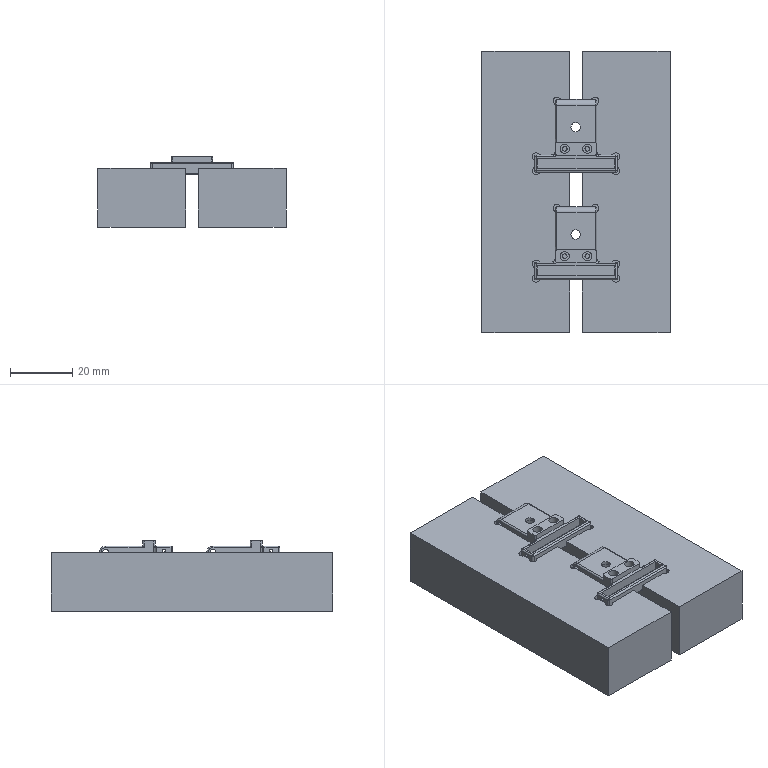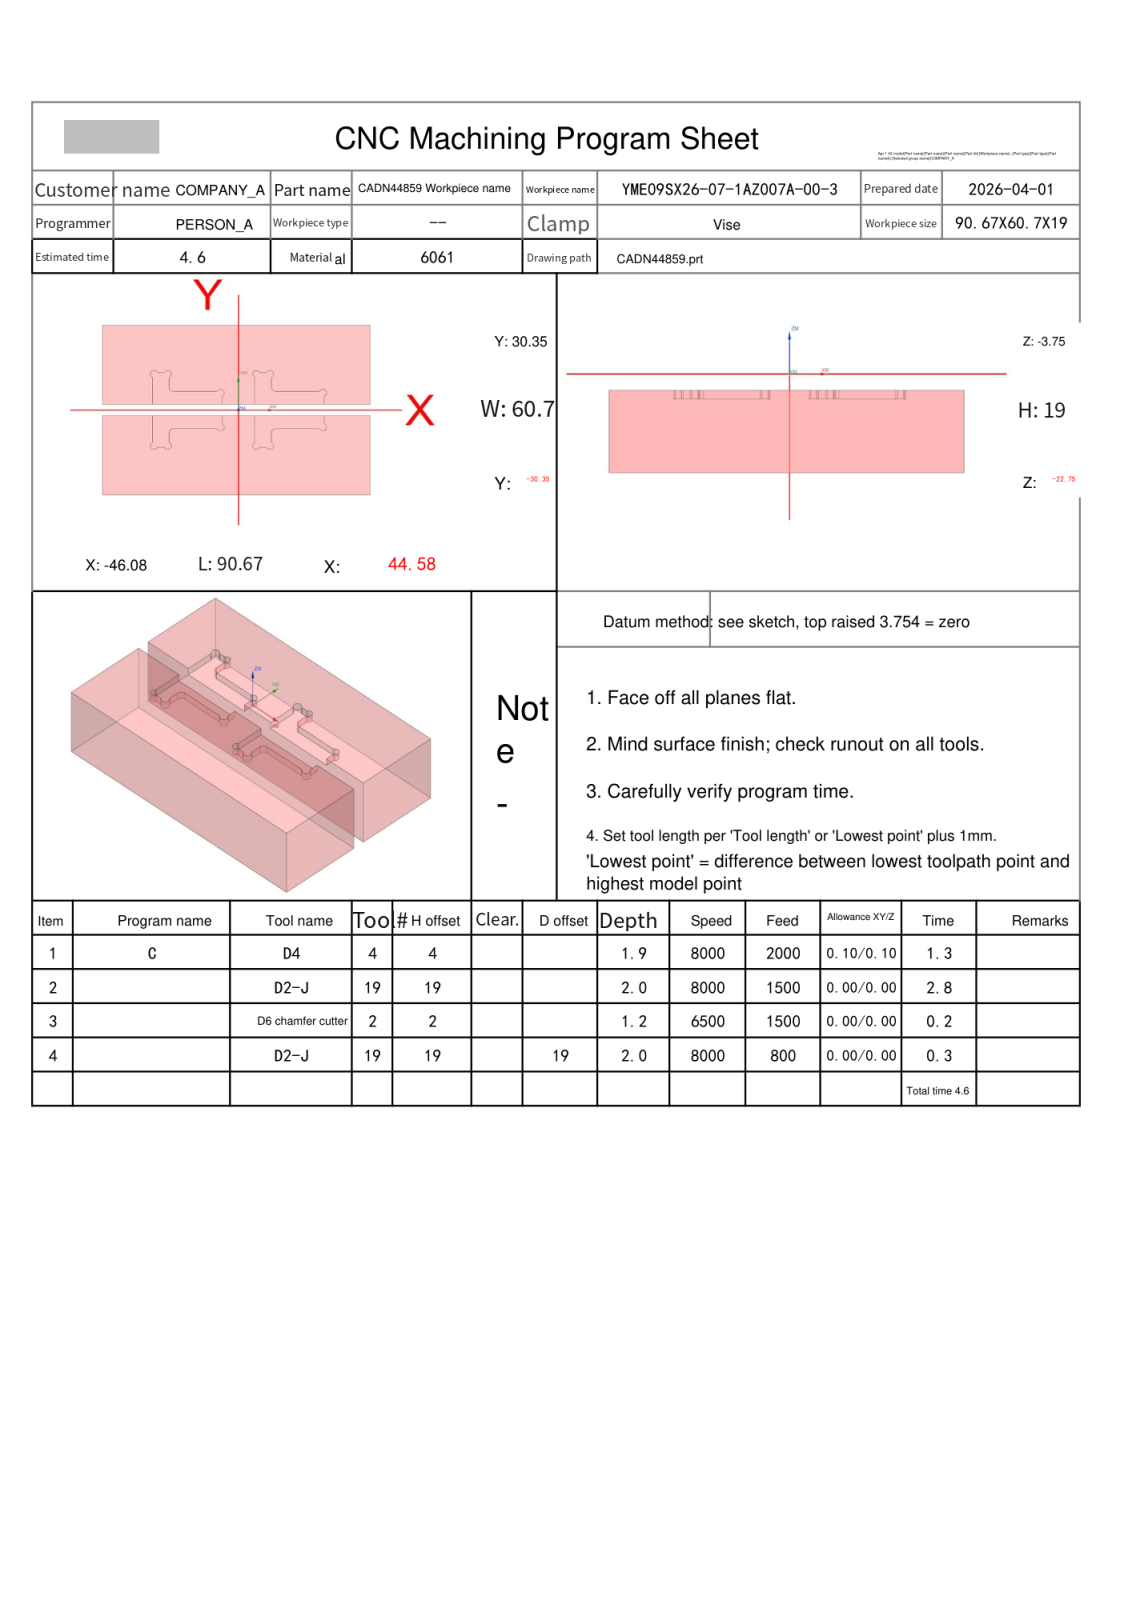NC program | NX | posted by the shop | part box 60.696 x 90.669 x 22.754 mm
Lines 1 to 949 of 8014:
%
O0001
(Machine time: 5.21 MIN)
(===Total Tool:3===)
(T4=D4      D=4.   R=0.   D-  H04 Z=-5.65 )
(T19=D2-J   D=2.   R=0.   D-  H19 Z=-5.75 )
(T2=D6 chamfer cutter   D=6.   R=0.   D-  H02 Z=-4.95 )
G80 G90 G17 G49 G40
G91 G28 Z0
M01
N1 T04 M06
(D4  D=4. R=0. H=04 ce=0.10 di=0.10)
G00 G90 G54 X-16.612 Y1.529 M03 S8000
G43 H04 Z6.346
M08
Z-2.254
G03 X-16.612 Y1.529 Z-2.847 I.128 J-1.795 F2000.
X-16.612 Y1.529 Z-3.439 I.128 J-1.795
X-16.484 Y1.534 Z-4.025 I.128 J-1.795
G01 X-21.952
G02 X-23.492 Y1.716 I0.0 J6.6
G01 X-23.584 Y1.727
G03 X-23.984 Y1.328 I0.0 J-.4
G01 Y-1.328
G03 X-23.584 Y-1.727 I.4 J.001
G01 X-23.492 Y-1.716
G02 X-21.952 Y-1.534 I1.54 J-6.418
G01 X-11.015
G03 X-10.616 Y-1.135 I-.001 J.4
G01 Y1.135
G03 X-11.015 Y1.534 I-.4 J-.001
G01 X-15.27
G02 X-15.602 Y1.712 I0.0 J.4
G01 X-17.365 Y4.356
G03 X-17.697 Y4.534 I-.333 J-.222
G01 X-21.952
G02 X-25.552 Y8.134 I0.0 J3.6
G01 Y11.248
X-26.984
Y3.819
G03 X-26.589 Y3.423 I.396 J0.0
G01 X-26.489 Y3.436
X-26.468 Y3.441
X-26.368 Y3.454
G02 X-26.013 Y3.238 I0.0 J-.4
G01 X-25.375 Y2.004
G03 X-24.487 Y1.463 I.888 J.459
X-23.487 Y2.463 I0.0 J1.
X-23.598 Y2.922 I-1. J0.0
G01 X-24.537 Y4.738
G03 X-25.425 Y5.279 I-.888 J-.459
X-26.422 Y4.365 I0.0 J-1.
G02 X-26.668 Y4.06 I-.348 J.03
G01 X-26.846 Y4.006
G03 X-26.984 Y3.819 I.057 J-.187
G01 Y-3.819
G03 X-26.846 Y-4.006 I.196 J0.0
G01 X-26.7 Y-4.051
G02 X-26.419 Y-4.389 I-.117 J-.383
G03 X-25.425 Y-5.279 I.994 J.11
X-24.537 Y-4.738 I0.0 J1.
G01 X-23.598 Y-2.922
G03 X-23.487 Y-2.463 I-.888 J.459
X-24.487 Y-1.463 I-1. J0.0
X-25.375 Y-2.004 I0.0 J-1.
G01 X-26.013 Y-3.238
G02 X-26.368 Y-3.454 I-.355 J.184
G01 X-26.468 Y-3.441
X-26.489 Y-3.436
X-26.589 Y-3.423
G03 X-26.984 Y-3.819 I0.0 J-.396
G01 Y-11.248
X-25.552
Y-8.134
G02 X-21.952 Y-4.534 I3.6 J0.0
G01 X-7.616
Y4.534
X-18.484
X-18.984
Y1.534
Z-2.525
G00 X-16.612 Y1.529
G03 X-16.612 Y1.529 Z-3.118 I.128 J-1.795
X-16.612 Y1.529 Z-3.711 I.128 J-1.795
X-16.484 Y1.534 Z-4.297 I.128 J-1.795
G01 X-21.952
G02 X-23.492 Y1.716 I0.0 J6.6
G01 X-23.584 Y1.727
G03 X-23.984 Y1.328 I0.0 J-.4
G01 Y-1.328
G03 X-23.584 Y-1.727 I.4 J.001
G01 X-23.492 Y-1.716
G02 X-21.952 Y-1.534 I1.54 J-6.418
G01 X-11.015
G03 X-10.616 Y-1.135 I-.001 J.4
G01 Y1.135
G03 X-11.015 Y1.534 I-.4 J-.001
G01 X-15.27
G02 X-15.602 Y1.712 I0.0 J.4
G01 X-17.365 Y4.356
G03 X-17.697 Y4.534 I-.333 J-.222
G01 X-21.952
G02 X-25.552 Y8.134 I0.0 J3.6
G01 Y11.248
X-26.984
Y3.819
G03 X-26.589 Y3.423 I.396 J0.0
G01 X-26.489 Y3.436
X-26.468 Y3.441
X-26.368 Y3.454
G02 X-26.013 Y3.238 I0.0 J-.4
G01 X-25.375 Y2.004
G03 X-24.487 Y1.463 I.888 J.459
X-23.487 Y2.463 I0.0 J1.
X-23.598 Y2.922 I-1. J0.0
G01 X-24.537 Y4.738
G03 X-25.425 Y5.279 I-.888 J-.459
X-26.422 Y4.365 I0.0 J-1.
G02 X-26.668 Y4.06 I-.348 J.03
G01 X-26.846 Y4.006
G03 X-26.984 Y3.819 I.057 J-.187
G01 Y-3.819
G03 X-26.846 Y-4.006 I.196 J0.0
G01 X-26.7 Y-4.051
G02 X-26.419 Y-4.389 I-.117 J-.383
G03 X-25.425 Y-5.279 I.994 J.11
X-24.537 Y-4.738 I0.0 J1.
G01 X-23.598 Y-2.922
G03 X-23.487 Y-2.463 I-.888 J.459
X-24.487 Y-1.463 I-1. J0.0
X-25.375 Y-2.004 I0.0 J-1.
G01 X-26.013 Y-3.238
G02 X-26.368 Y-3.454 I-.355 J.184
G01 X-26.468 Y-3.441
X-26.489 Y-3.436
X-26.589 Y-3.423
G03 X-26.984 Y-3.819 I0.0 J-.396
G01 Y-11.248
X-25.552
Y-8.134
G02 X-21.952 Y-4.534 I3.6 J0.0
G01 X-7.616
Y4.534
X-18.484
X-18.984
Y1.534
Z-2.797
G00 X-16.612 Y1.529
G03 X-16.612 Y1.529 Z-3.39 I.128 J-1.795
X-16.612 Y1.529 Z-3.982 I.128 J-1.795
X-16.484 Y1.534 Z-4.568 I.128 J-1.795
G01 X-21.952
G02 X-23.492 Y1.716 I0.0 J6.6
G01 X-23.584 Y1.727
G03 X-23.984 Y1.328 I0.0 J-.4
G01 Y-1.328
G03 X-23.584 Y-1.727 I.4 J.001
G01 X-23.492 Y-1.716
G02 X-21.952 Y-1.534 I1.54 J-6.418
G01 X-11.015
G03 X-10.616 Y-1.135 I-.001 J.4
G01 Y1.135
G03 X-11.015 Y1.534 I-.4 J-.001
G01 X-15.27
G02 X-15.602 Y1.712 I0.0 J.4
G01 X-17.365 Y4.356
G03 X-17.697 Y4.534 I-.333 J-.222
G01 X-21.952
G02 X-25.552 Y8.134 I0.0 J3.6
G01 Y11.248
X-26.984
Y3.819
G03 X-26.589 Y3.423 I.396 J0.0
G01 X-26.489 Y3.436
X-26.468 Y3.441
X-26.368 Y3.454
G02 X-26.013 Y3.238 I0.0 J-.4
G01 X-25.375 Y2.004
G03 X-24.487 Y1.463 I.888 J.459
X-23.487 Y2.463 I0.0 J1.
X-23.598 Y2.922 I-1. J0.0
G01 X-24.537 Y4.738
G03 X-25.425 Y5.279 I-.888 J-.459
X-26.422 Y4.365 I0.0 J-1.
G02 X-26.668 Y4.06 I-.348 J.03
G01 X-26.846 Y4.006
G03 X-26.984 Y3.819 I.057 J-.187
G01 Y-3.819
G03 X-26.846 Y-4.006 I.196 J0.0
G01 X-26.7 Y-4.051
G02 X-26.419 Y-4.389 I-.117 J-.383
G03 X-25.425 Y-5.279 I.994 J.11
X-24.537 Y-4.738 I0.0 J1.
G01 X-23.598 Y-2.922
G03 X-23.487 Y-2.463 I-.888 J.459
X-24.487 Y-1.463 I-1. J0.0
X-25.375 Y-2.004 I0.0 J-1.
G01 X-26.013 Y-3.238
G02 X-26.368 Y-3.454 I-.355 J.184
G01 X-26.468 Y-3.441
X-26.489 Y-3.436
X-26.589 Y-3.423
G03 X-26.984 Y-3.819 I0.0 J-.396
G01 Y-11.248
X-25.552
Y-8.134
G02 X-21.952 Y-4.534 I3.6 J0.0
G01 X-7.616
Y4.534
X-18.484
X-18.984
Y1.534
Z-3.068
G00 X-16.612 Y1.529
G03 X-16.612 Y1.529 Z-3.661 I.128 J-1.795
X-16.612 Y1.529 Z-4.254 I.128 J-1.795
X-16.484 Y1.534 Z-4.84 I.128 J-1.795
G01 X-21.952
G02 X-23.492 Y1.716 I0.0 J6.6
G01 X-23.584 Y1.727
G03 X-23.984 Y1.328 I0.0 J-.4
G01 Y-1.328
G03 X-23.584 Y-1.727 I.4 J.001
G01 X-23.492 Y-1.716
G02 X-21.952 Y-1.534 I1.54 J-6.418
G01 X-11.015
G03 X-10.616 Y-1.135 I-.001 J.4
G01 Y1.135
G03 X-11.015 Y1.534 I-.4 J-.001
G01 X-15.27
G02 X-15.602 Y1.712 I0.0 J.4
G01 X-17.365 Y4.356
G03 X-17.697 Y4.534 I-.333 J-.222
G01 X-21.952
G02 X-25.552 Y8.134 I0.0 J3.6
G01 Y11.248
X-26.984
Y3.819
G03 X-26.589 Y3.423 I.396 J0.0
G01 X-26.489 Y3.436
X-26.468 Y3.441
X-26.368 Y3.454
G02 X-26.013 Y3.238 I0.0 J-.4
G01 X-25.375 Y2.004
G03 X-24.487 Y1.463 I.888 J.459
X-23.487 Y2.463 I0.0 J1.
X-23.598 Y2.922 I-1. J0.0
G01 X-24.537 Y4.738
G03 X-25.425 Y5.279 I-.888 J-.459
X-26.422 Y4.365 I0.0 J-1.
G02 X-26.668 Y4.06 I-.348 J.03
G01 X-26.846 Y4.006
G03 X-26.984 Y3.819 I.057 J-.187
G01 Y-3.819
G03 X-26.846 Y-4.006 I.196 J0.0
G01 X-26.7 Y-4.051
G02 X-26.419 Y-4.389 I-.117 J-.383
G03 X-25.425 Y-5.279 I.994 J.11
X-24.537 Y-4.738 I0.0 J1.
G01 X-23.598 Y-2.922
G03 X-23.487 Y-2.463 I-.888 J.459
X-24.487 Y-1.463 I-1. J0.0
X-25.375 Y-2.004 I0.0 J-1.
G01 X-26.013 Y-3.238
G02 X-26.368 Y-3.454 I-.355 J.184
G01 X-26.468 Y-3.441
X-26.489 Y-3.436
X-26.589 Y-3.423
G03 X-26.984 Y-3.819 I0.0 J-.396
G01 Y-11.248
X-25.552
Y-8.134
G02 X-21.952 Y-4.534 I3.6 J0.0
G01 X-7.616
Y4.534
X-18.484
X-18.984
Y1.534
Z-3.34
G00 X-16.612 Y1.529
G03 X-16.612 Y1.529 Z-3.932 I.128 J-1.795
X-16.612 Y1.529 Z-4.525 I.128 J-1.795
X-16.484 Y1.534 Z-5.111 I.128 J-1.795
G01 X-21.952
G02 X-23.492 Y1.716 I0.0 J6.6
G01 X-23.584 Y1.727
G03 X-23.984 Y1.328 I0.0 J-.4
G01 Y-1.328
G03 X-23.584 Y-1.727 I.4 J.001
G01 X-23.492 Y-1.716
G02 X-21.952 Y-1.534 I1.54 J-6.418
G01 X-11.015
G03 X-10.616 Y-1.135 I-.001 J.4
G01 Y1.135
G03 X-11.015 Y1.534 I-.4 J-.001
G01 X-15.27
G02 X-15.602 Y1.712 I0.0 J.4
G01 X-17.365 Y4.356
G03 X-17.697 Y4.534 I-.333 J-.222
G01 X-21.952
G02 X-25.552 Y8.134 I0.0 J3.6
G01 Y11.248
X-26.984
Y3.819
G03 X-26.589 Y3.423 I.396 J0.0
G01 X-26.489 Y3.436
X-26.468 Y3.441
X-26.368 Y3.454
G02 X-26.013 Y3.238 I0.0 J-.4
G01 X-25.375 Y2.004
G03 X-24.487 Y1.463 I.888 J.459
X-23.487 Y2.463 I0.0 J1.
X-23.598 Y2.922 I-1. J0.0
G01 X-24.537 Y4.738
G03 X-25.425 Y5.279 I-.888 J-.459
X-26.422 Y4.365 I0.0 J-1.
G02 X-26.668 Y4.06 I-.348 J.03
G01 X-26.846 Y4.006
G03 X-26.984 Y3.819 I.057 J-.187
G01 Y-3.819
G03 X-26.846 Y-4.006 I.196 J0.0
G01 X-26.7 Y-4.051
G02 X-26.419 Y-4.389 I-.117 J-.383
G03 X-25.425 Y-5.279 I.994 J.11
X-24.537 Y-4.738 I0.0 J1.
G01 X-23.598 Y-2.922
G03 X-23.487 Y-2.463 I-.888 J.459
X-24.487 Y-1.463 I-1. J0.0
X-25.375 Y-2.004 I0.0 J-1.
G01 X-26.013 Y-3.238
G02 X-26.368 Y-3.454 I-.355 J.184
G01 X-26.468 Y-3.441
X-26.489 Y-3.436
X-26.589 Y-3.423
G03 X-26.984 Y-3.819 I0.0 J-.396
G01 Y-11.248
X-25.552
Y-8.134
G02 X-21.952 Y-4.534 I3.6 J0.0
G01 X-7.616
Y4.534
X-18.484
X-18.984
Y1.534
Z-3.611
G00 X-16.612 Y1.529
G03 X-16.612 Y1.529 Z-4.204 I.128 J-1.795
X-16.612 Y1.529 Z-4.797 I.128 J-1.795
X-16.484 Y1.534 Z-5.383 I.128 J-1.795
G01 X-21.952
G02 X-23.492 Y1.716 I0.0 J6.6
G01 X-23.584 Y1.727
G03 X-23.984 Y1.328 I0.0 J-.4
G01 Y-1.328
G03 X-23.584 Y-1.727 I.4 J.001
G01 X-23.492 Y-1.716
G02 X-21.952 Y-1.534 I1.54 J-6.418
G01 X-11.015
G03 X-10.616 Y-1.135 I-.001 J.4
G01 Y1.135
G03 X-11.015 Y1.534 I-.4 J-.001
G01 X-15.27
G02 X-15.602 Y1.712 I0.0 J.4
G01 X-17.365 Y4.356
G03 X-17.697 Y4.534 I-.333 J-.222
G01 X-21.952
G02 X-25.552 Y8.134 I0.0 J3.6
G01 Y11.248
X-26.984
Y3.819
G03 X-26.589 Y3.423 I.396 J0.0
G01 X-26.489 Y3.436
X-26.468 Y3.441
X-26.368 Y3.454
G02 X-26.013 Y3.238 I0.0 J-.4
G01 X-25.375 Y2.004
G03 X-24.487 Y1.463 I.888 J.459
X-23.487 Y2.463 I0.0 J1.
X-23.598 Y2.922 I-1. J0.0
G01 X-24.537 Y4.738
G03 X-25.425 Y5.279 I-.888 J-.459
X-26.422 Y4.365 I0.0 J-1.
G02 X-26.668 Y4.06 I-.348 J.03
G01 X-26.846 Y4.006
G03 X-26.984 Y3.819 I.057 J-.187
G01 Y-3.819
G03 X-26.846 Y-4.006 I.196 J0.0
G01 X-26.7 Y-4.051
G02 X-26.419 Y-4.389 I-.117 J-.383
G03 X-25.425 Y-5.279 I.994 J.11
X-24.537 Y-4.738 I0.0 J1.
G01 X-23.598 Y-2.922
G03 X-23.487 Y-2.463 I-.888 J.459
X-24.487 Y-1.463 I-1. J0.0
X-25.375 Y-2.004 I0.0 J-1.
G01 X-26.013 Y-3.238
G02 X-26.368 Y-3.454 I-.355 J.184
G01 X-26.468 Y-3.441
X-26.489 Y-3.436
X-26.589 Y-3.423
G03 X-26.984 Y-3.819 I0.0 J-.396
G01 Y-11.248
X-25.552
Y-8.134
G02 X-21.952 Y-4.534 I3.6 J0.0
G01 X-7.616
Y4.534
X-18.484
X-18.984
Y1.534
Z-3.883
G00 X-16.612 Y1.529
G03 X-16.612 Y1.529 Z-4.475 I.128 J-1.795
X-16.612 Y1.529 Z-5.068 I.128 J-1.795
X-16.484 Y1.534 Z-5.654 I.128 J-1.795
G01 X-21.952
G02 X-23.492 Y1.716 I0.0 J6.6
G01 X-23.584 Y1.727
G03 X-23.984 Y1.328 I0.0 J-.4
G01 Y-1.328
G03 X-23.584 Y-1.727 I.4 J.001
G01 X-23.492 Y-1.716
G02 X-21.952 Y-1.534 I1.54 J-6.418
G01 X-11.015
G03 X-10.616 Y-1.135 I-.001 J.4
G01 Y1.135
G03 X-11.015 Y1.534 I-.4 J-.001
G01 X-15.27
G02 X-15.602 Y1.712 I0.0 J.4
G01 X-17.365 Y4.356
G03 X-17.697 Y4.534 I-.333 J-.222
G01 X-21.952
G02 X-25.552 Y8.134 I0.0 J3.6
G01 Y11.248
X-26.984
Y3.819
G03 X-26.589 Y3.423 I.396 J0.0
G01 X-26.489 Y3.436
X-26.468 Y3.441
X-26.368 Y3.454
G02 X-26.013 Y3.238 I0.0 J-.4
G01 X-25.375 Y2.004
G03 X-24.487 Y1.463 I.888 J.459
X-23.487 Y2.463 I0.0 J1.
X-23.598 Y2.922 I-1. J0.0
G01 X-24.537 Y4.738
G03 X-25.425 Y5.279 I-.888 J-.459
X-26.422 Y4.365 I0.0 J-1.
G02 X-26.668 Y4.06 I-.348 J.03
G01 X-26.846 Y4.006
G03 X-26.984 Y3.819 I.057 J-.187
G01 Y-3.819
G03 X-26.846 Y-4.006 I.196 J0.0
G01 X-26.7 Y-4.051
G02 X-26.419 Y-4.389 I-.117 J-.383
G03 X-25.425 Y-5.279 I.994 J.11
X-24.537 Y-4.738 I0.0 J1.
G01 X-23.598 Y-2.922
G03 X-23.487 Y-2.463 I-.888 J.459
X-24.487 Y-1.463 I-1. J0.0
X-25.375 Y-2.004 I0.0 J-1.
G01 X-26.013 Y-3.238
G02 X-26.368 Y-3.454 I-.355 J.184
G01 X-26.468 Y-3.441
X-26.489 Y-3.436
X-26.589 Y-3.423
G03 X-26.984 Y-3.819 I0.0 J-.396
G01 Y-11.248
X-25.552
Y-8.134
G02 X-21.952 Y-4.534 I3.6 J0.0
G01 X-7.616
Y4.534
X-18.484
X-18.984
Y1.534
Z-4.154
G00 Z6.346
X17.988 Y1.529
Z-2.254
G03 X17.988 Y1.529 Z-2.847 I.128 J-1.795
X17.988 Y1.529 Z-3.439 I.128 J-1.795
X18.116 Y1.534 Z-4.025 I.128 J-1.795
G01 X12.648
G02 X11.108 Y1.716 I0.0 J6.6
G01 X11.016 Y1.727
G03 X10.616 Y1.328 I0.0 J-.4
G01 Y-1.328
G03 X11.016 Y-1.727 I.4 J.001
G01 X11.108 Y-1.716
G02 X12.648 Y-1.534 I1.54 J-6.418
G01 X23.585
G03 X23.984 Y-1.135 I-.001 J.4
G01 Y1.135
G03 X23.585 Y1.534 I-.4 J-.001
G01 X19.33
G02 X18.998 Y1.712 I0.0 J.4
G01 X17.235 Y4.356
G03 X16.903 Y4.534 I-.333 J-.222
G01 X12.648
G02 X9.048 Y8.134 I0.0 J3.6
G01 Y11.248
X7.616
Y3.819
G03 X8.011 Y3.423 I.396 J0.0
G01 X8.111 Y3.436
X8.132 Y3.441
X8.232 Y3.454
G02 X8.587 Y3.238 I0.0 J-.4
G01 X9.225 Y2.004
G03 X10.113 Y1.463 I.888 J.459
X11.113 Y2.463 I0.0 J1.
X11.002 Y2.922 I-1. J0.0
G01 X10.063 Y4.738
G03 X9.175 Y5.279 I-.888 J-.459
X8.178 Y4.365 I0.0 J-1.
G02 X7.932 Y4.06 I-.348 J.03
G01 X7.754 Y4.006
G03 X7.616 Y3.819 I.057 J-.187
G01 Y-3.819
G03 X7.754 Y-4.006 I.196 J0.0
G01 X7.9 Y-4.051
G02 X8.181 Y-4.389 I-.117 J-.383
G03 X9.175 Y-5.279 I.994 J.11
X10.063 Y-4.738 I0.0 J1.
G01 X11.002 Y-2.922
G03 X11.113 Y-2.463 I-.888 J.459
X10.113 Y-1.463 I-1. J0.0
X9.225 Y-2.004 I0.0 J-1.
G01 X8.587 Y-3.238
G02 X8.232 Y-3.454 I-.355 J.184
G01 X8.132 Y-3.441
X8.111 Y-3.436
X8.011 Y-3.423
G03 X7.616 Y-3.819 I0.0 J-.396
G01 Y-11.248
X9.048
Y-8.134
G02 X12.648 Y-4.534 I3.6 J0.0
G01 X26.984
Y4.534
X16.116
X15.616
Y1.534
Z-2.525
G00 X17.988 Y1.529
G03 X17.988 Y1.529 Z-3.118 I.128 J-1.795
X17.988 Y1.529 Z-3.711 I.128 J-1.795
X18.116 Y1.534 Z-4.297 I.128 J-1.795
G01 X12.648
G02 X11.108 Y1.716 I0.0 J6.6
G01 X11.016 Y1.727
G03 X10.616 Y1.328 I0.0 J-.4
G01 Y-1.328
G03 X11.016 Y-1.727 I.4 J.001
G01 X11.108 Y-1.716
G02 X12.648 Y-1.534 I1.54 J-6.418
G01 X23.585
G03 X23.984 Y-1.135 I-.001 J.4
G01 Y1.135
G03 X23.585 Y1.534 I-.4 J-.001
G01 X19.33
G02 X18.998 Y1.712 I0.0 J.4
G01 X17.235 Y4.356
G03 X16.903 Y4.534 I-.333 J-.222
G01 X12.648
G02 X9.048 Y8.134 I0.0 J3.6
G01 Y11.248
X7.616
Y3.819
G03 X8.011 Y3.423 I.396 J0.0
G01 X8.111 Y3.436
X8.132 Y3.441
X8.232 Y3.454
G02 X8.587 Y3.238 I0.0 J-.4
G01 X9.225 Y2.004
G03 X10.113 Y1.463 I.888 J.459
X11.113 Y2.463 I0.0 J1.
X11.002 Y2.922 I-1. J0.0
G01 X10.063 Y4.738
G03 X9.175 Y5.279 I-.888 J-.459
X8.178 Y4.365 I0.0 J-1.
G02 X7.932 Y4.06 I-.348 J.03
G01 X7.754 Y4.006
G03 X7.616 Y3.819 I.057 J-.187
G01 Y-3.819
G03 X7.754 Y-4.006 I.196 J0.0
G01 X7.9 Y-4.051
G02 X8.181 Y-4.389 I-.117 J-.383
G03 X9.175 Y-5.279 I.994 J.11
X10.063 Y-4.738 I0.0 J1.
G01 X11.002 Y-2.922
G03 X11.113 Y-2.463 I-.888 J.459
X10.113 Y-1.463 I-1. J0.0
X9.225 Y-2.004 I0.0 J-1.
G01 X8.587 Y-3.238
G02 X8.232 Y-3.454 I-.355 J.184
G01 X8.132 Y-3.441
X8.111 Y-3.436
X8.011 Y-3.423
G03 X7.616 Y-3.819 I0.0 J-.396
G01 Y-11.248
X9.048
Y-8.134
G02 X12.648 Y-4.534 I3.6 J0.0
G01 X26.984
Y4.534
X16.116
X15.616
Y1.534
Z-2.797
G00 X17.988 Y1.529
G03 X17.988 Y1.529 Z-3.39 I.128 J-1.795
X17.988 Y1.529 Z-3.982 I.128 J-1.795
X18.116 Y1.534 Z-4.568 I.128 J-1.795
G01 X12.648
G02 X11.108 Y1.716 I0.0 J6.6
G01 X11.016 Y1.727
G03 X10.616 Y1.328 I0.0 J-.4
G01 Y-1.328
G03 X11.016 Y-1.727 I.4 J.001
G01 X11.108 Y-1.716
G02 X12.648 Y-1.534 I1.54 J-6.418
G01 X23.585
G03 X23.984 Y-1.135 I-.001 J.4
G01 Y1.135
G03 X23.585 Y1.534 I-.4 J-.001
G01 X19.33
G02 X18.998 Y1.712 I0.0 J.4
G01 X17.235 Y4.356
G03 X16.903 Y4.534 I-.333 J-.222
G01 X12.648
G02 X9.048 Y8.134 I0.0 J3.6
G01 Y11.248
X7.616
Y3.819
G03 X8.011 Y3.423 I.396 J0.0
G01 X8.111 Y3.436
X8.132 Y3.441
X8.232 Y3.454
G02 X8.587 Y3.238 I0.0 J-.4
G01 X9.225 Y2.004
G03 X10.113 Y1.463 I.888 J.459
X11.113 Y2.463 I0.0 J1.
X11.002 Y2.922 I-1. J0.0
G01 X10.063 Y4.738
G03 X9.175 Y5.279 I-.888 J-.459
X8.178 Y4.365 I0.0 J-1.
G02 X7.932 Y4.06 I-.348 J.03
G01 X7.754 Y4.006
G03 X7.616 Y3.819 I.057 J-.187
G01 Y-3.819
G03 X7.754 Y-4.006 I.196 J0.0
G01 X7.9 Y-4.051
G02 X8.181 Y-4.389 I-.117 J-.383
G03 X9.175 Y-5.279 I.994 J.11
X10.063 Y-4.738 I0.0 J1.
G01 X11.002 Y-2.922
G03 X11.113 Y-2.463 I-.888 J.459
X10.113 Y-1.463 I-1. J0.0
X9.225 Y-2.004 I0.0 J-1.
G01 X8.587 Y-3.238
G02 X8.232 Y-3.454 I-.355 J.184
G01 X8.132 Y-3.441
X8.111 Y-3.436
X8.011 Y-3.423
G03 X7.616 Y-3.819 I0.0 J-.396
G01 Y-11.248
X9.048
Y-8.134
G02 X12.648 Y-4.534 I3.6 J0.0
G01 X26.984
Y4.534
X16.116
X15.616
Y1.534
Z-3.068
G00 X17.988 Y1.529
G03 X17.988 Y1.529 Z-3.661 I.128 J-1.795
X17.988 Y1.529 Z-4.254 I.128 J-1.795
X18.116 Y1.534 Z-4.84 I.128 J-1.795
G01 X12.648
G02 X11.108 Y1.716 I0.0 J6.6
G01 X11.016 Y1.727
G03 X10.616 Y1.328 I0.0 J-.4
G01 Y-1.328
G03 X11.016 Y-1.727 I.4 J.001
G01 X11.108 Y-1.716
G02 X12.648 Y-1.534 I1.54 J-6.418
G01 X23.585
G03 X23.984 Y-1.135 I-.001 J.4
G01 Y1.135
G03 X23.585 Y1.534 I-.4 J-.001
G01 X19.33
G02 X18.998 Y1.712 I0.0 J.4
G01 X17.235 Y4.356
G03 X16.903 Y4.534 I-.333 J-.222
G01 X12.648
G02 X9.048 Y8.134 I0.0 J3.6
G01 Y11.248
X7.616
Y3.819
G03 X8.011 Y3.423 I.396 J0.0
G01 X8.111 Y3.436
X8.132 Y3.441
X8.232 Y3.454
G02 X8.587 Y3.238 I0.0 J-.4
G01 X9.225 Y2.004
G03 X10.113 Y1.463 I.888 J.459
X11.113 Y2.463 I0.0 J1.
X11.002 Y2.922 I-1. J0.0
G01 X10.063 Y4.738
G03 X9.175 Y5.279 I-.888 J-.459
X8.178 Y4.365 I0.0 J-1.
G02 X7.932 Y4.06 I-.348 J.03
G01 X7.754 Y4.006
G03 X7.616 Y3.819 I.057 J-.187
G01 Y-3.819
G03 X7.754 Y-4.006 I.196 J0.0
G01 X7.9 Y-4.051
G02 X8.181 Y-4.389 I-.117 J-.383
G03 X9.175 Y-5.279 I.994 J.11
X10.063 Y-4.738 I0.0 J1.
G01 X11.002 Y-2.922
G03 X11.113 Y-2.463 I-.888 J.459
X10.113 Y-1.463 I-1. J0.0
X9.225 Y-2.004 I0.0 J-1.
G01 X8.587 Y-3.238
G02 X8.232 Y-3.454 I-.355 J.184
G01 X8.132 Y-3.441
X8.111 Y-3.436
X8.011 Y-3.423
G03 X7.616 Y-3.819 I0.0 J-.396
G01 Y-11.248
X9.048
Y-8.134
G02 X12.648 Y-4.534 I3.6 J0.0
G01 X26.984
Y4.534
X16.116
X15.616
Y1.534
Z-3.34
G00 X17.988 Y1.529
G03 X17.988 Y1.529 Z-3.932 I.128 J-1.795
X17.988 Y1.529 Z-4.525 I.128 J-1.795
X18.116 Y1.534 Z-5.111 I.128 J-1.795
G01 X12.648
G02 X11.108 Y1.716 I0.0 J6.6
G01 X11.016 Y1.727
G03 X10.616 Y1.328 I0.0 J-.4
G01 Y-1.328
G03 X11.016 Y-1.727 I.4 J.001
G01 X11.108 Y-1.716
G02 X12.648 Y-1.534 I1.54 J-6.418
G01 X23.585
G03 X23.984 Y-1.135 I-.001 J.4
G01 Y1.135
G03 X23.585 Y1.534 I-.4 J-.001
G01 X19.33
G02 X18.998 Y1.712 I0.0 J.4
G01 X17.235 Y4.356
G03 X16.903 Y4.534 I-.333 J-.222
G01 X12.648
G02 X9.048 Y8.134 I0.0 J3.6
G01 Y11.248
X7.616
Y3.819
G03 X8.011 Y3.423 I.396 J0.0
G01 X8.111 Y3.436
X8.132 Y3.441
X8.232 Y3.454
G02 X8.587 Y3.238 I0.0 J-.4
G01 X9.225 Y2.004
G03 X10.113 Y1.463 I.888 J.459
X11.113 Y2.463 I0.0 J1.
X11.002 Y2.922 I-1. J0.0
G01 X10.063 Y4.738
G03 X9.175 Y5.279 I-.888 J-.459
X8.178 Y4.365 I0.0 J-1.
G02 X7.932 Y4.06 I-.348 J.03
G01 X7.754 Y4.006
G03 X7.616 Y3.819 I.057 J-.187
G01 Y-3.819
G03 X7.754 Y-4.006 I.196 J0.0
G01 X7.9 Y-4.051
G02 X8.181 Y-4.389 I-.117 J-.383
G03 X9.175 Y-5.279 I.994 J.11
X10.063 Y-4.738 I0.0 J1.
G01 X11.002 Y-2.922
G03 X11.113 Y-2.463 I-.888 J.459
X10.113 Y-1.463 I-1. J0.0
X9.225 Y-2.004 I0.0 J-1.
G01 X8.587 Y-3.238
G02 X8.232 Y-3.454 I-.355 J.184
G01 X8.132 Y-3.441
X8.111 Y-3.436
X8.011 Y-3.423
G03 X7.616 Y-3.819 I0.0 J-.396
G01 Y-11.248
X9.048
Y-8.134
G02 X12.648 Y-4.534 I3.6 J0.0
G01 X26.984
Y4.534
X16.116
X15.616
Y1.534
Z-3.611
G00 X17.988 Y1.529
G03 X17.988 Y1.529 Z-4.204 I.128 J-1.795
X17.988 Y1.529 Z-4.797 I.128 J-1.795
X18.116 Y1.534 Z-5.383 I.128 J-1.795
G01 X12.648
G02 X11.108 Y1.716 I0.0 J6.6
G01 X11.016 Y1.727
G03 X10.616 Y1.328 I0.0 J-.4
G01 Y-1.328
G03 X11.016 Y-1.727 I.4 J.001
G01 X11.108 Y-1.716
G02 X12.648 Y-1.534 I1.54 J-6.418
G01 X23.585
G03 X23.984 Y-1.135 I-.001 J.4
G01 Y1.135
G03 X23.585 Y1.534 I-.4 J-.001
G01 X19.33
G02 X18.998 Y1.712 I0.0 J.4
G01 X17.235 Y4.356
G03 X16.903 Y4.534 I-.333 J-.222
G01 X12.648
G02 X9.048 Y8.134 I0.0 J3.6
G01 Y11.248
X7.616
Y3.819
G03 X8.011 Y3.423 I.396 J0.0
G01 X8.111 Y3.436
X8.132 Y3.441
X8.232 Y3.454
G02 X8.587 Y3.238 I0.0 J-.4
G01 X9.225 Y2.004
G03 X10.113 Y1.463 I.888 J.459
X11.113 Y2.463 I0.0 J1.
X11.002 Y2.922 I-1. J0.0
G01 X10.063 Y4.738
G03 X9.175 Y5.279 I-.888 J-.459
X8.178 Y4.365 I0.0 J-1.
G02 X7.932 Y4.06 I-.348 J.03
G01 X7.754 Y4.006
G03 X7.616 Y3.819 I.057 J-.187
G01 Y-3.819
G03 X7.754 Y-4.006 I.196 J0.0
G01 X7.9 Y-4.051
G02 X8.181 Y-4.389 I-.117 J-.383
G03 X9.175 Y-5.279 I.994 J.11
X10.063 Y-4.738 I0.0 J1.
G01 X11.002 Y-2.922
G03 X11.113 Y-2.463 I-.888 J.459
X10.113 Y-1.463 I-1. J0.0
X9.225 Y-2.004 I0.0 J-1.
G01 X8.587 Y-3.238
G02 X8.232 Y-3.454 I-.355 J.184
G01 X8.132 Y-3.441
X8.111 Y-3.436
X8.011 Y-3.423
G03 X7.616 Y-3.819 I0.0 J-.396
G01 Y-11.248
X9.048
Y-8.134
G02 X12.648 Y-4.534 I3.6 J0.0
G01 X26.984
Y4.534
X16.116
X15.616
Y1.534
Z-3.883
G00 X17.988 Y1.529
G03 X17.988 Y1.529 Z-4.475 I.128 J-1.795
X17.988 Y1.529 Z-5.068 I.128 J-1.795
X18.116 Y1.534 Z-5.654 I.128 J-1.795
G01 X12.648
G02 X11.108 Y1.716 I0.0 J6.6
G01 X11.016 Y1.727
G03 X10.616 Y1.328 I0.0 J-.4
G01 Y-1.328
G03 X11.016 Y-1.727 I.4 J.001
G01 X11.108 Y-1.716
G02 X12.648 Y-1.534 I1.54 J-6.418
G01 X23.585
G03 X23.984 Y-1.135 I-.001 J.4
G01 Y1.135
G03 X23.585 Y1.534 I-.4 J-.001
G01 X19.33
G02 X18.998 Y1.712 I0.0 J.4
G01 X17.235 Y4.356
G03 X16.903 Y4.534 I-.333 J-.222
G01 X12.648
G02 X9.048 Y8.134 I0.0 J3.6
G01 Y11.248
X7.616
Y3.819
G03 X8.011 Y3.423 I.396 J0.0
G01 X8.111 Y3.436
X8.132 Y3.441
X8.232 Y3.454
G02 X8.587 Y3.238 I0.0 J-.4
G01 X9.225 Y2.004
G03 X10.113 Y1.463 I.888 J.459
X11.113 Y2.463 I0.0 J1.
X11.002 Y2.922 I-1. J0.0
G01 X10.063 Y4.738
G03 X9.175 Y5.279 I-.888 J-.459
X8.178 Y4.365 I0.0 J-1.
G02 X7.932 Y4.06 I-.348 J.03
G01 X7.754 Y4.006
G03 X7.616 Y3.819 I.057 J-.187
G01 Y-3.819
G03 X7.754 Y-4.006 I.196 J0.0
G01 X7.9 Y-4.051
G02 X8.181 Y-4.389 I-.117 J-.383
G03 X9.175 Y-5.279 I.994 J.11
X10.063 Y-4.738 I0.0 J1.
G01 X11.002 Y-2.922
G03 X11.113 Y-2.463 I-.888 J.459
X10.113 Y-1.463 I-1. J0.0
X9.225 Y-2.004 I0.0 J-1.
G01 X8.587 Y-3.238
G02 X8.232 Y-3.454 I-.355 J.184
G01 X8.132 Y-3.441
X8.111 Y-3.436
X8.011 Y-3.423
G03 X7.616 Y-3.819 I0.0 J-.396
G01 Y-11.248
X9.048
Y-8.134
G02 X12.648 Y-4.534 I3.6 J0.0
G01 X26.984
Y4.534
X16.116
X15.616
Y1.534
Z-4.154
G00 Z6.346
G91 G28 Z0.0
M05
M09
G91 G28 Z0.0
M01